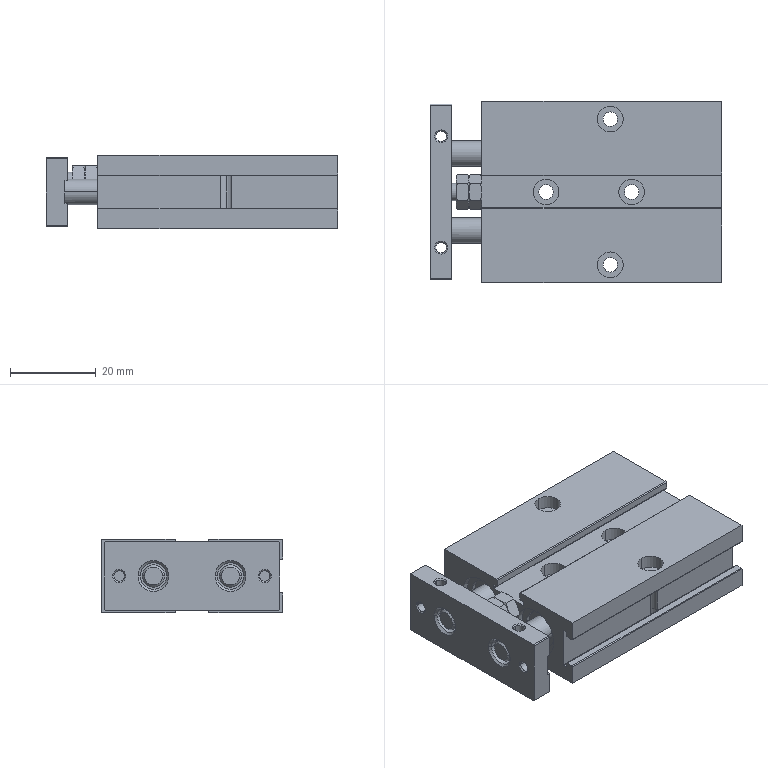Part | SolidWorks | 2 solids | 266 faces | box 68 x 42.3 x 17.2 mm | volume 37108 mm3 | cylinder 106 | plane 100 | cone 60 | commonest cylinder face diameters 0.4 x26 6 x24 2.459 x8 3.4 x8 9 x8 10 x8